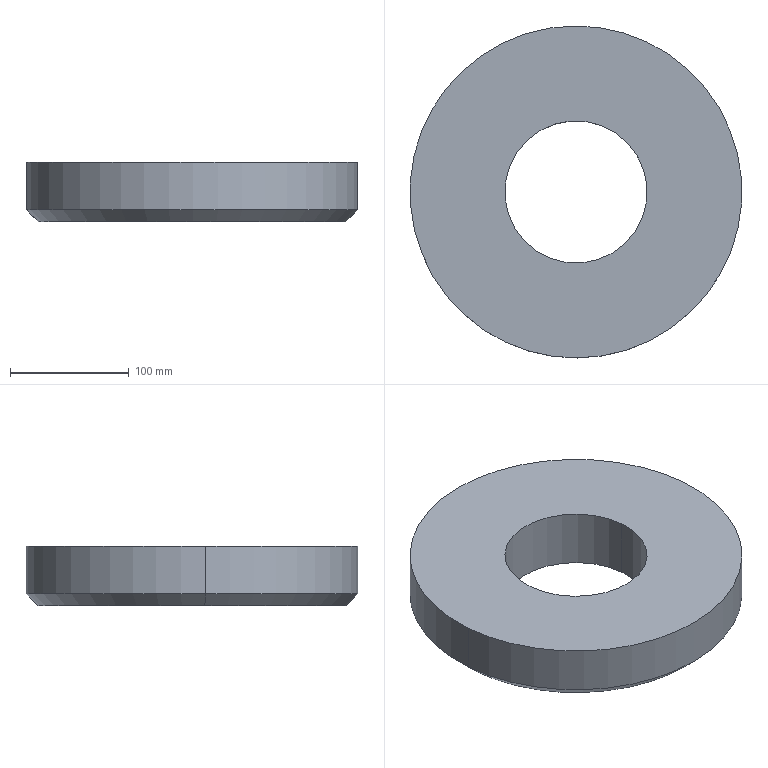Part | SolidWorks | features BaseBody 1 | 1 solid | 8 faces | box 280 x 280 x 50 mm | volume 2470339 mm3 | cylinder 4 | cone 2 | plane 2 | commonest cylinder face diameters 120 x2 280 x2
STEP:
#1=CARTESIAN_POINT('',(404.594,964.868,-924.893));
#2=VERTEX_POINT('',#1);
#3=CARTESIAN_POINT('',(394.628,964.038,-934.893));
#4=VERTEX_POINT('',#3);
#5=CARTESIAN_POINT('',(404.594,964.868,-924.893));
#6=DIRECTION('',(-0.7047,-0.05869,-0.7071));
#7=VECTOR('',#6,1000.);
#8=LINE('',#5,#7);
#9=EDGE_CURVE('',#2,#4,#8,.T.);
#10=ORIENTED_EDGE('',*,*,#9,.T.);
#11=CARTESIAN_POINT('',(135.525,942.459,-934.893));
#12=VERTEX_POINT('',#11);
#13=CARTESIAN_POINT('',(265.077,953.249,-934.893));
#14=DIRECTION('',(0.,0.,-1.));
#15=DIRECTION('',(-0.9965,-0.083,0.));
#16=AXIS2_PLACEMENT_3D('',#13,#14,#15);
#17=CIRCLE('',#16,130.);
#18=EDGE_CURVE('',#12,#4,#17,.T.);
#19=ORIENTED_EDGE('',*,*,#18,.F.);
#20=CARTESIAN_POINT('',(125.56,941.63,-924.893));
#21=VERTEX_POINT('',#20);
#22=CARTESIAN_POINT('',(125.56,941.63,-924.893));
#23=DIRECTION('',(0.7047,0.05869,-0.7071));
#24=VECTOR('',#23,1000.);
#25=LINE('',#22,#24);
#26=EDGE_CURVE('',#21,#12,#25,.T.);
#27=ORIENTED_EDGE('',*,*,#26,.F.);
#28=CARTESIAN_POINT('',(265.077,953.249,-924.893));
#29=DIRECTION('',(0.,0.,1.));
#30=DIRECTION('',(-0.9965,-0.083,0.));
#31=AXIS2_PLACEMENT_3D('',#28,#29,#30);
#32=CIRCLE('',#31,140.);
#33=EDGE_CURVE('',#2,#21,#32,.T.);
#34=ORIENTED_EDGE('',*,*,#33,.F.);
#35=EDGE_LOOP('',(#10,#19,#27,#34));
#36=FACE_OUTER_BOUND('',#35,.T.);
#37=CARTESIAN_POINT('',(265.077,953.249,-924.893));
#38=DIRECTION('',(0.,0.,1.));
#39=DIRECTION('',(0.9965,0.083,0.));
#40=AXIS2_PLACEMENT_3D('',#37,#38,#39);
#41=CONICAL_SURFACE('',#40,140.,0.7854);
#42=ADVANCED_FACE('',(#36),#41,.T.);
#43=CARTESIAN_POINT('',(205.284,948.269,-934.893));
#44=VERTEX_POINT('',#43);
#45=CARTESIAN_POINT('',(205.284,948.269,-884.893));
#46=VERTEX_POINT('',#45);
#47=CARTESIAN_POINT('',(205.284,948.269,-884.893));
#48=DIRECTION('',(0.,0.,1.));
#49=VECTOR('',#48,1000.);
#50=LINE('',#47,#49);
#51=EDGE_CURVE('',#44,#46,#50,.T.);
#52=ORIENTED_EDGE('',*,*,#51,.T.);
#53=CARTESIAN_POINT('',(324.87,958.229,-884.893));
#54=VERTEX_POINT('',#53);
#55=CARTESIAN_POINT('',(265.077,953.249,-884.893));
#56=DIRECTION('',(0.,0.,1.));
#57=DIRECTION('',(-0.9965,-0.083,0.));
#58=AXIS2_PLACEMENT_3D('',#55,#56,#57);
#59=CIRCLE('',#58,60.);
#60=EDGE_CURVE('',#46,#54,#59,.T.);
#61=ORIENTED_EDGE('',*,*,#60,.T.);
#62=CARTESIAN_POINT('',(324.87,958.229,-934.893));
#63=VERTEX_POINT('',#62);
#64=CARTESIAN_POINT('',(324.87,958.229,-884.893));
#65=DIRECTION('',(0.,0.,1.));
#66=VECTOR('',#65,1000.);
#67=LINE('',#64,#66);
#68=EDGE_CURVE('',#63,#54,#67,.T.);
#69=ORIENTED_EDGE('',*,*,#68,.F.);
#70=CARTESIAN_POINT('',(265.077,953.249,-934.893));
#71=DIRECTION('',(0.,0.,1.));
#72=DIRECTION('',(-0.9965,-0.083,0.));
#73=AXIS2_PLACEMENT_3D('',#70,#71,#72);
#74=CIRCLE('',#73,60.);
#75=EDGE_CURVE('',#44,#63,#74,.T.);
#76=ORIENTED_EDGE('',*,*,#75,.F.);
#77=EDGE_LOOP('',(#52,#61,#69,#76));
#78=FACE_OUTER_BOUND('',#77,.T.);
#79=CARTESIAN_POINT('',(265.077,953.249,-884.893));
#80=DIRECTION('',(0.,0.,-1.));
#81=DIRECTION('',(-0.9965,-0.083,0.));
#82=AXIS2_PLACEMENT_3D('',#79,#80,#81);
#83=CYLINDRICAL_SURFACE('',#82,60.);
#84=ADVANCED_FACE('',(#78),#83,.F.);
#85=CARTESIAN_POINT('',(125.56,941.63,-884.893));
#86=VERTEX_POINT('',#85);
#87=CARTESIAN_POINT('',(125.56,941.63,-884.893));
#88=DIRECTION('',(0.,0.,1.));
#89=VECTOR('',#88,1000.);
#90=LINE('',#87,#89);
#91=EDGE_CURVE('',#21,#86,#90,.T.);
#92=ORIENTED_EDGE('',*,*,#91,.T.);
#93=CARTESIAN_POINT('',(404.594,964.868,-884.893));
#94=VERTEX_POINT('',#93);
#95=CARTESIAN_POINT('',(265.077,953.249,-884.893));
#96=DIRECTION('',(0.,0.,1.));
#97=DIRECTION('',(-0.9965,-0.083,0.));
#98=AXIS2_PLACEMENT_3D('',#95,#96,#97);
#99=CIRCLE('',#98,140.);
#100=EDGE_CURVE('',#94,#86,#99,.T.);
#101=ORIENTED_EDGE('',*,*,#100,.F.);
#102=CARTESIAN_POINT('',(404.594,964.868,-884.893));
#103=DIRECTION('',(0.,0.,1.));
#104=VECTOR('',#103,1000.);
#105=LINE('',#102,#104);
#106=EDGE_CURVE('',#2,#94,#105,.T.);
#107=ORIENTED_EDGE('',*,*,#106,.F.);
#108=ORIENTED_EDGE('',*,*,#33,.T.);
#109=EDGE_LOOP('',(#92,#101,#107,#108));
#110=FACE_OUTER_BOUND('',#109,.T.);
#111=CARTESIAN_POINT('',(265.077,953.249,-884.893));
#112=DIRECTION('',(0.,0.,-1.));
#113=DIRECTION('',(-0.9965,-0.083,0.));
#114=AXIS2_PLACEMENT_3D('',#111,#112,#113);
#115=CYLINDRICAL_SURFACE('',#114,140.);
#116=ADVANCED_FACE('',(#110),#115,.T.);
#117=CARTESIAN_POINT('',(265.077,953.249,-934.893));
#118=DIRECTION('',(0.,0.,1.));
#119=DIRECTION('',(-0.9965,-0.083,0.));
#120=AXIS2_PLACEMENT_3D('',#117,#118,#119);
#121=CIRCLE('',#120,60.);
#122=EDGE_CURVE('',#63,#44,#121,.T.);
#123=ORIENTED_EDGE('',*,*,#122,.T.);
#124=ORIENTED_EDGE('',*,*,#75,.T.);
#125=EDGE_LOOP('',(#123,#124));
#126=FACE_BOUND('',#125,.T.);
#127=ORIENTED_EDGE('',*,*,#18,.T.);
#128=CARTESIAN_POINT('',(265.077,953.249,-934.893));
#129=DIRECTION('',(0.,0.,-1.));
#130=DIRECTION('',(-0.9965,-0.083,0.));
#131=AXIS2_PLACEMENT_3D('',#128,#129,#130);
#132=CIRCLE('',#131,130.);
#133=EDGE_CURVE('',#4,#12,#132,.T.);
#134=ORIENTED_EDGE('',*,*,#133,.T.);
#135=EDGE_LOOP('',(#127,#134));
#136=FACE_OUTER_BOUND('',#135,.T.);
#137=CARTESIAN_POINT('',(265.077,953.249,-934.893));
#138=DIRECTION('',(0.,0.,1.));
#139=DIRECTION('',(1.,0.,0.));
#140=AXIS2_PLACEMENT_3D('',#137,#138,#139);
#141=PLANE('',#140);
#142=ADVANCED_FACE('',(#126,#136),#141,.F.);
#143=CARTESIAN_POINT('',(265.077,953.249,-884.893));
#144=DIRECTION('',(0.,0.,1.));
#145=DIRECTION('',(-0.9965,-0.083,0.));
#146=AXIS2_PLACEMENT_3D('',#143,#144,#145);
#147=CIRCLE('',#146,60.);
#148=EDGE_CURVE('',#54,#46,#147,.T.);
#149=ORIENTED_EDGE('',*,*,#148,.F.);
#150=ORIENTED_EDGE('',*,*,#60,.F.);
#151=EDGE_LOOP('',(#149,#150));
#152=FACE_BOUND('',#151,.T.);
#153=ORIENTED_EDGE('',*,*,#100,.T.);
#154=CARTESIAN_POINT('',(265.077,953.249,-884.893));
#155=DIRECTION('',(0.,0.,1.));
#156=DIRECTION('',(-0.9965,-0.083,0.));
#157=AXIS2_PLACEMENT_3D('',#154,#155,#156);
#158=CIRCLE('',#157,140.);
#159=EDGE_CURVE('',#86,#94,#158,.T.);
#160=ORIENTED_EDGE('',*,*,#159,.T.);
#161=EDGE_LOOP('',(#153,#160));
#162=FACE_OUTER_BOUND('',#161,.T.);
#163=CARTESIAN_POINT('',(265.077,953.249,-884.893));
#164=DIRECTION('',(0.,0.,1.));
#165=DIRECTION('',(1.,0.,0.));
#166=AXIS2_PLACEMENT_3D('',#163,#164,#165);
#167=PLANE('',#166);
#168=ADVANCED_FACE('',(#152,#162),#167,.T.);
#169=ORIENTED_EDGE('',*,*,#159,.F.);
#170=ORIENTED_EDGE('',*,*,#91,.F.);
#171=CARTESIAN_POINT('',(265.077,953.249,-924.893));
#172=DIRECTION('',(0.,0.,1.));
#173=DIRECTION('',(-0.9965,-0.083,0.));
#174=AXIS2_PLACEMENT_3D('',#171,#172,#173);
#175=CIRCLE('',#174,140.);
#176=EDGE_CURVE('',#21,#2,#175,.T.);
#177=ORIENTED_EDGE('',*,*,#176,.T.);
#178=ORIENTED_EDGE('',*,*,#106,.T.);
#179=EDGE_LOOP('',(#169,#170,#177,#178));
#180=FACE_OUTER_BOUND('',#179,.T.);
#181=CARTESIAN_POINT('',(265.077,953.249,-884.893));
#182=DIRECTION('',(0.,0.,-1.));
#183=DIRECTION('',(-0.9965,-0.083,0.));
#184=AXIS2_PLACEMENT_3D('',#181,#182,#183);
#185=CYLINDRICAL_SURFACE('',#184,140.);
#186=ADVANCED_FACE('',(#180),#185,.T.);
#187=ORIENTED_EDGE('',*,*,#148,.T.);
#188=ORIENTED_EDGE('',*,*,#51,.F.);
#189=ORIENTED_EDGE('',*,*,#122,.F.);
#190=ORIENTED_EDGE('',*,*,#68,.T.);
#191=EDGE_LOOP('',(#187,#188,#189,#190));
#192=FACE_OUTER_BOUND('',#191,.T.);
#193=CARTESIAN_POINT('',(265.077,953.249,-884.893));
#194=DIRECTION('',(0.,0.,-1.));
#195=DIRECTION('',(-0.9965,-0.083,0.));
#196=AXIS2_PLACEMENT_3D('',#193,#194,#195);
#197=CYLINDRICAL_SURFACE('',#196,60.);
#198=ADVANCED_FACE('',(#192),#197,.F.);
#199=ORIENTED_EDGE('',*,*,#133,.F.);
#200=ORIENTED_EDGE('',*,*,#9,.F.);
#201=ORIENTED_EDGE('',*,*,#176,.F.);
#202=ORIENTED_EDGE('',*,*,#26,.T.);
#203=EDGE_LOOP('',(#199,#200,#201,#202));
#204=FACE_OUTER_BOUND('',#203,.T.);
#205=CARTESIAN_POINT('',(265.077,953.249,-924.893));
#206=DIRECTION('',(0.,0.,1.));
#207=DIRECTION('',(0.9965,0.083,0.));
#208=AXIS2_PLACEMENT_3D('',#205,#206,#207);
#209=CONICAL_SURFACE('',#208,140.,0.7854);
#210=ADVANCED_FACE('',(#204),#209,.T.);
#211=CLOSED_SHELL('',(#42,#84,#116,#142,#168,#186,#198,#210));
#212=MANIFOLD_SOLID_BREP('',#211);
#213=CARTESIAN_POINT('',(0.,0.,0.));
#214=DIRECTION('',(0.,0.,1.));
#215=DIRECTION('',(1.,0.,0.));
#216=AXIS2_PLACEMENT_3D('',#213,#214,#215);
#217=(LENGTH_UNIT()NAMED_UNIT(*)SI_UNIT(.MILLI.,.METRE.));
#218=UNCERTAINTY_MEASURE_WITH_UNIT(LENGTH_MEASURE(0.00001),#217,'','');
#219=(NAMED_UNIT(*)PLANE_ANGLE_UNIT()SI_UNIT($,.RADIAN.));
#220=(NAMED_UNIT(*)SI_UNIT($,.STERADIAN.)SOLID_ANGLE_UNIT());
#221=(GEOMETRIC_REPRESENTATION_CONTEXT(3)GLOBAL_UNCERTAINTY_ASSIGNED_CONTEXT((#218))GLOBAL_UNIT_ASSIGNED_CONTEXT((#217,#219,#220))REPRESENTATION_CONTEXT('',''));
#222=ADVANCED_BREP_SHAPE_REPRESENTATION('',(#212,#216),#221);